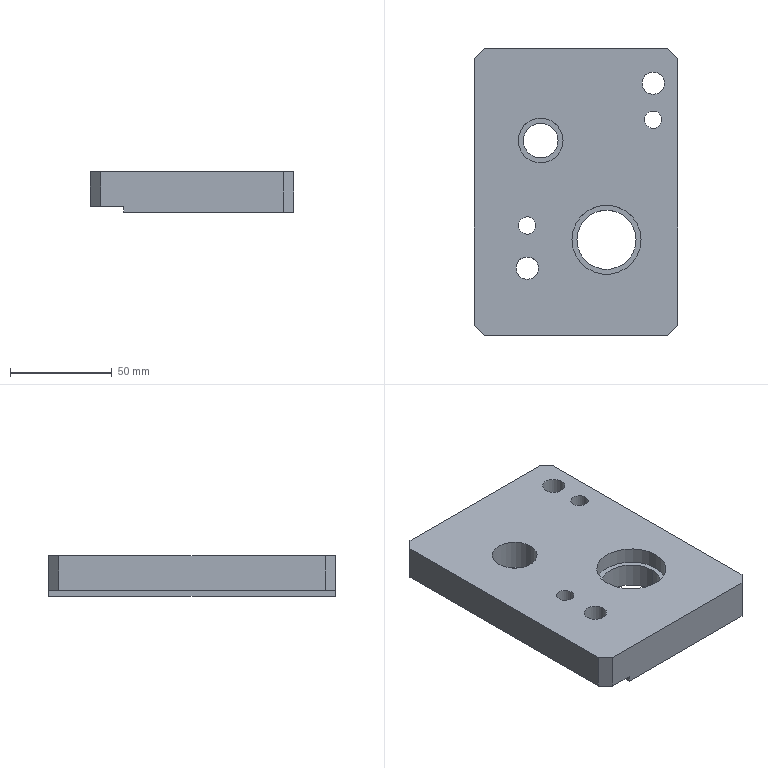Part | STEP file | lll_id3050_x_t | 1 solid | 32 faces | box 100 x 141 x 20 mm | volume 242474 mm3 | plane 18 | cylinder 14 | commonest cylinder face diameters 11 x4 8.5 x2 17 x2 17.07 x2 29.07 x2 22 x1
STEP:
#1=CARTESIAN_POINT('',(3254.117,-145.288,22.5));
#2=VERTEX_POINT('',#1);
#3=CARTESIAN_POINT('',(3258.367,-145.288,22.5));
#4=DIRECTION('',(0.,0.,1.));
#5=DIRECTION('',(-1.,0.,0.));
#6=AXIS2_PLACEMENT_3D('',#3,#4,#5);
#7=CIRCLE('',#6,4.25);
#8=EDGE_CURVE('',#2,#2,#7,.T.);
#9=ORIENTED_EDGE('',*,*,#8,.F.);
#10=EDGE_LOOP('',(#9));
#11=FACE_BOUND('',#10,.T.);
#12=CARTESIAN_POINT('',(3192.117,-197.288,22.5));
#13=VERTEX_POINT('',#12);
#14=CARTESIAN_POINT('',(3196.367,-197.288,22.5));
#15=DIRECTION('',(0.,0.,1.));
#16=DIRECTION('',(-1.,0.,0.));
#17=AXIS2_PLACEMENT_3D('',#14,#15,#16);
#18=CIRCLE('',#17,4.25);
#19=EDGE_CURVE('',#13,#13,#18,.T.);
#20=ORIENTED_EDGE('',*,*,#19,.F.);
#21=EDGE_LOOP('',(#20));
#22=FACE_BOUND('',#21,.T.);
#23=CARTESIAN_POINT('',(3252.867,-127.288,22.5));
#24=VERTEX_POINT('',#23);
#25=CARTESIAN_POINT('',(3258.367,-127.288,22.5));
#26=DIRECTION('',(0.,0.,1.));
#27=DIRECTION('',(-1.,0.,0.));
#28=AXIS2_PLACEMENT_3D('',#25,#26,#27);
#29=CIRCLE('',#28,5.5);
#30=EDGE_CURVE('',#24,#24,#29,.T.);
#31=ORIENTED_EDGE('',*,*,#30,.F.);
#32=EDGE_LOOP('',(#31));
#33=FACE_BOUND('',#32,.T.);
#34=CARTESIAN_POINT('',(3175.367,-110.288,22.5));
#35=VERTEX_POINT('',#34);
#36=CARTESIAN_POINT('',(3265.367,-110.288,22.5));
#37=VERTEX_POINT('',#36);
#38=CARTESIAN_POINT('',(3227.867,-110.288,22.5));
#39=DIRECTION('',(1.,0.,0.));
#40=VECTOR('',#39,1.);
#41=LINE('',#38,#40);
#42=EDGE_CURVE('',#35,#37,#41,.T.);
#43=ORIENTED_EDGE('',*,*,#42,.F.);
#44=CARTESIAN_POINT('',(3170.367,-115.288,22.5));
#45=VERTEX_POINT('',#44);
#46=CARTESIAN_POINT('',(3328.404,42.749,22.5));
#47=DIRECTION('',(-0.7071,-0.7071,0.));
#48=VECTOR('',#47,1.);
#49=LINE('',#46,#48);
#50=EDGE_CURVE('',#35,#45,#49,.T.);
#51=ORIENTED_EDGE('',*,*,#50,.T.);
#52=CARTESIAN_POINT('',(3170.367,-246.288,22.5));
#53=VERTEX_POINT('',#52);
#54=CARTESIAN_POINT('',(3170.367,-166.13,22.5));
#55=DIRECTION('',(0.,-1.,0.));
#56=VECTOR('',#55,1.);
#57=LINE('',#54,#56);
#58=EDGE_CURVE('',#45,#53,#57,.T.);
#59=ORIENTED_EDGE('',*,*,#58,.T.);
#60=CARTESIAN_POINT('',(3175.367,-251.288,22.5));
#61=VERTEX_POINT('',#60);
#62=CARTESIAN_POINT('',(3313.747,-389.668,22.5));
#63=DIRECTION('',(0.7071,-0.7071,0.));
#64=VECTOR('',#63,1.);
#65=LINE('',#62,#64);
#66=EDGE_CURVE('',#53,#61,#65,.T.);
#67=ORIENTED_EDGE('',*,*,#66,.T.);
#68=CARTESIAN_POINT('',(3265.367,-251.288,22.5));
#69=VERTEX_POINT('',#68);
#70=CARTESIAN_POINT('',(3227.867,-251.288,22.5));
#71=DIRECTION('',(-1.,0.,0.));
#72=VECTOR('',#71,1.);
#73=LINE('',#70,#72);
#74=EDGE_CURVE('',#69,#61,#73,.T.);
#75=ORIENTED_EDGE('',*,*,#74,.F.);
#76=CARTESIAN_POINT('',(3270.367,-246.288,22.5));
#77=VERTEX_POINT('',#76);
#78=CARTESIAN_POINT('',(3443.904,-72.751,22.5));
#79=DIRECTION('',(0.7071,0.7071,0.));
#80=VECTOR('',#79,1.);
#81=LINE('',#78,#80);
#82=EDGE_CURVE('',#69,#77,#81,.T.);
#83=ORIENTED_EDGE('',*,*,#82,.T.);
#84=CARTESIAN_POINT('',(3270.367,-115.288,22.5));
#85=VERTEX_POINT('',#84);
#86=CARTESIAN_POINT('',(3270.367,-195.288,22.5));
#87=DIRECTION('',(0.,-1.,0.));
#88=VECTOR('',#87,1.);
#89=LINE('',#86,#88);
#90=EDGE_CURVE('',#85,#77,#89,.T.);
#91=ORIENTED_EDGE('',*,*,#90,.F.);
#92=CARTESIAN_POINT('',(3429.247,-274.168,22.5));
#93=DIRECTION('',(-0.7071,0.7071,0.));
#94=VECTOR('',#93,1.);
#95=LINE('',#92,#94);
#96=EDGE_CURVE('',#85,#37,#95,.T.);
#97=ORIENTED_EDGE('',*,*,#96,.T.);
#98=EDGE_LOOP('',(#43,#51,#59,#67,#75,#83,#91,#97));
#99=FACE_BOUND('',#98,.T.);
#100=CARTESIAN_POINT('',(3190.867,-218.288,22.5));
#101=VERTEX_POINT('',#100);
#102=CARTESIAN_POINT('',(3196.367,-218.288,22.5));
#103=DIRECTION('',(0.,0.,1.));
#104=DIRECTION('',(-1.,0.,0.));
#105=AXIS2_PLACEMENT_3D('',#102,#103,#104);
#106=CIRCLE('',#105,5.5);
#107=EDGE_CURVE('',#101,#101,#106,.T.);
#108=ORIENTED_EDGE('',*,*,#107,.F.);
#109=EDGE_LOOP('',(#108));
#110=FACE_BOUND('',#109,.T.);
#111=CARTESIAN_POINT('',(3214.,-155.5,22.5));
#112=VERTEX_POINT('',#111);
#113=CARTESIAN_POINT('',(3203.,-155.5,22.5));
#114=DIRECTION('',(0.,0.,1.));
#115=DIRECTION('',(1.,0.,0.));
#116=AXIS2_PLACEMENT_3D('',#113,#114,#115);
#117=CIRCLE('',#116,11.);
#118=EDGE_CURVE('',#112,#112,#117,.T.);
#119=ORIENTED_EDGE('',*,*,#118,.F.);
#120=EDGE_LOOP('',(#119));
#121=FACE_BOUND('',#120,.T.);
#122=CARTESIAN_POINT('',(3252.367,-204.288,22.5));
#123=VERTEX_POINT('',#122);
#124=CARTESIAN_POINT('',(3235.367,-204.288,22.5));
#125=DIRECTION('',(0.,0.,-1.));
#126=DIRECTION('',(1.,0.,0.));
#127=AXIS2_PLACEMENT_3D('',#124,#125,#126);
#128=CIRCLE('',#127,17.);
#129=EDGE_CURVE('',#123,#123,#128,.T.);
#130=ORIENTED_EDGE('',*,*,#129,.T.);
#131=EDGE_LOOP('',(#130));
#132=FACE_BOUND('',#131,.T.);
#133=CARTESIAN_POINT('',(3537.284,-166.13,22.5));
#134=DIRECTION('',(0.,0.,1.));
#135=DIRECTION('',(0.,1.,0.));
#136=AXIS2_PLACEMENT_3D('',#133,#134,#135);
#137=PLANE('',#136);
#138=ADVANCED_FACE('',(#11,#22,#33,#99,#110,#121,#132),#137,.T.);
#139=CARTESIAN_POINT('',(3190.867,-197.288,2.5));
#140=VERTEX_POINT('',#139);
#141=CARTESIAN_POINT('',(3196.367,-197.288,2.5));
#142=DIRECTION('',(0.,0.,1.));
#143=DIRECTION('',(-1.,0.,0.));
#144=AXIS2_PLACEMENT_3D('',#141,#142,#143);
#145=CIRCLE('',#144,5.5);
#146=EDGE_CURVE('',#140,#140,#145,.T.);
#147=ORIENTED_EDGE('',*,*,#146,.T.);
#148=EDGE_LOOP('',(#147));
#149=FACE_BOUND('',#148,.T.);
#150=CARTESIAN_POINT('',(3187.867,-218.288,2.5));
#151=VERTEX_POINT('',#150);
#152=CARTESIAN_POINT('',(3196.367,-218.288,2.5));
#153=DIRECTION('',(0.,0.,1.));
#154=DIRECTION('',(-1.,0.,0.));
#155=AXIS2_PLACEMENT_3D('',#152,#153,#154);
#156=CIRCLE('',#155,8.5);
#157=EDGE_CURVE('',#151,#151,#156,.T.);
#158=ORIENTED_EDGE('',*,*,#157,.T.);
#159=EDGE_LOOP('',(#158));
#160=FACE_BOUND('',#159,.T.);
#161=CARTESIAN_POINT('',(3211.535,-155.5,2.5));
#162=VERTEX_POINT('',#161);
#163=CARTESIAN_POINT('',(3194.465,-155.5,2.5));
#164=VERTEX_POINT('',#163);
#165=CARTESIAN_POINT('',(3203.,-155.5,2.5));
#166=DIRECTION('',(0.,0.,-1.));
#167=DIRECTION('',(-1.,0.,0.));
#168=AXIS2_PLACEMENT_3D('',#165,#166,#167);
#169=CIRCLE('',#168,8.535);
#170=EDGE_CURVE('',#162,#164,#169,.T.);
#171=ORIENTED_EDGE('',*,*,#170,.F.);
#172=CARTESIAN_POINT('',(3203.,-155.5,2.5));
#173=DIRECTION('',(0.,0.,-1.));
#174=DIRECTION('',(-1.,0.,0.));
#175=AXIS2_PLACEMENT_3D('',#172,#173,#174);
#176=CIRCLE('',#175,8.535);
#177=EDGE_CURVE('',#164,#162,#176,.T.);
#178=ORIENTED_EDGE('',*,*,#177,.F.);
#179=EDGE_LOOP('',(#171,#178));
#180=FACE_BOUND('',#179,.T.);
#181=CARTESIAN_POINT('',(3249.902,-204.288,2.5));
#182=VERTEX_POINT('',#181);
#183=CARTESIAN_POINT('',(3220.832,-204.288,2.5));
#184=VERTEX_POINT('',#183);
#185=CARTESIAN_POINT('',(3235.367,-204.288,2.5));
#186=DIRECTION('',(0.,0.,-1.));
#187=DIRECTION('',(-1.,0.,0.));
#188=AXIS2_PLACEMENT_3D('',#185,#186,#187);
#189=CIRCLE('',#188,14.535);
#190=EDGE_CURVE('',#182,#184,#189,.T.);
#191=ORIENTED_EDGE('',*,*,#190,.F.);
#192=CARTESIAN_POINT('',(3235.367,-204.288,2.5));
#193=DIRECTION('',(0.,0.,-1.));
#194=DIRECTION('',(-1.,0.,0.));
#195=AXIS2_PLACEMENT_3D('',#192,#193,#194);
#196=CIRCLE('',#195,14.535);
#197=EDGE_CURVE('',#184,#182,#196,.T.);
#198=ORIENTED_EDGE('',*,*,#197,.F.);
#199=EDGE_LOOP('',(#191,#198));
#200=FACE_BOUND('',#199,.T.);
#201=CARTESIAN_POINT('',(3249.867,-127.288,2.5));
#202=VERTEX_POINT('',#201);
#203=CARTESIAN_POINT('',(3258.367,-127.288,2.5));
#204=DIRECTION('',(0.,0.,-1.));
#205=DIRECTION('',(-1.,0.,0.));
#206=AXIS2_PLACEMENT_3D('',#203,#204,#205);
#207=CIRCLE('',#206,8.5);
#208=EDGE_CURVE('',#202,#202,#207,.T.);
#209=ORIENTED_EDGE('',*,*,#208,.F.);
#210=EDGE_LOOP('',(#209));
#211=FACE_BOUND('',#210,.T.);
#212=CARTESIAN_POINT('',(3252.867,-145.288,2.5));
#213=VERTEX_POINT('',#212);
#214=CARTESIAN_POINT('',(3258.367,-145.288,2.5));
#215=DIRECTION('',(0.,0.,-1.));
#216=DIRECTION('',(-1.,0.,0.));
#217=AXIS2_PLACEMENT_3D('',#214,#215,#216);
#218=CIRCLE('',#217,5.5);
#219=EDGE_CURVE('',#213,#213,#218,.T.);
#220=ORIENTED_EDGE('',*,*,#219,.F.);
#221=EDGE_LOOP('',(#220));
#222=FACE_BOUND('',#221,.T.);
#223=CARTESIAN_POINT('',(3265.367,-110.288,2.5));
#224=VERTEX_POINT('',#223);
#225=CARTESIAN_POINT('',(3186.89,-110.288,2.5));
#226=VERTEX_POINT('',#225);
#227=CARTESIAN_POINT('',(2132.435,-110.288,2.5));
#228=DIRECTION('',(-1.,0.,0.));
#229=VECTOR('',#228,1.);
#230=LINE('',#227,#229);
#231=EDGE_CURVE('',#224,#226,#230,.T.);
#232=ORIENTED_EDGE('',*,*,#231,.F.);
#233=CARTESIAN_POINT('',(3270.367,-115.288,2.5));
#234=VERTEX_POINT('',#233);
#235=CARTESIAN_POINT('',(3270.367,-115.288,2.5));
#236=DIRECTION('',(0.7071,-0.7071,0.));
#237=VECTOR('',#236,1.);
#238=LINE('',#235,#237);
#239=EDGE_CURVE('',#224,#234,#238,.T.);
#240=ORIENTED_EDGE('',*,*,#239,.T.);
#241=CARTESIAN_POINT('',(3270.367,-246.288,2.5));
#242=VERTEX_POINT('',#241);
#243=CARTESIAN_POINT('',(3270.367,0.,2.5));
#244=DIRECTION('',(0.,1.,0.));
#245=VECTOR('',#244,1.);
#246=LINE('',#243,#245);
#247=EDGE_CURVE('',#242,#234,#246,.T.);
#248=ORIENTED_EDGE('',*,*,#247,.F.);
#249=CARTESIAN_POINT('',(3265.367,-251.288,2.5));
#250=VERTEX_POINT('',#249);
#251=CARTESIAN_POINT('',(3265.367,-251.288,2.5));
#252=DIRECTION('',(-0.7071,-0.7071,0.));
#253=VECTOR('',#252,1.);
#254=LINE('',#251,#253);
#255=EDGE_CURVE('',#242,#250,#254,.T.);
#256=ORIENTED_EDGE('',*,*,#255,.T.);
#257=CARTESIAN_POINT('',(3186.89,-251.288,2.5));
#258=VERTEX_POINT('',#257);
#259=CARTESIAN_POINT('',(2132.435,-251.288,2.5));
#260=DIRECTION('',(1.,0.,0.));
#261=VECTOR('',#260,1.);
#262=LINE('',#259,#261);
#263=EDGE_CURVE('',#258,#250,#262,.T.);
#264=ORIENTED_EDGE('',*,*,#263,.F.);
#265=CARTESIAN_POINT('',(3186.89,-185.788,2.5));
#266=DIRECTION('',(0.,-1.,0.));
#267=VECTOR('',#266,1.);
#268=LINE('',#265,#267);
#269=EDGE_CURVE('',#226,#258,#268,.T.);
#270=ORIENTED_EDGE('',*,*,#269,.F.);
#271=EDGE_LOOP('',(#232,#240,#248,#256,#264,#270));
#272=FACE_BOUND('',#271,.T.);
#273=CARTESIAN_POINT('',(2132.435,0.,2.5));
#274=DIRECTION('',(0.,0.,-1.));
#275=DIRECTION('',(-1.,0.,0.));
#276=AXIS2_PLACEMENT_3D('',#273,#274,#275);
#277=PLANE('',#276);
#278=ADVANCED_FACE('',(#149,#160,#180,#200,#211,#222,#272),#277,.T.);
#279=CARTESIAN_POINT('',(3190.867,-197.288,9.5));
#280=VERTEX_POINT('',#279);
#281=CARTESIAN_POINT('',(3196.367,-197.288,9.5));
#282=DIRECTION('',(0.,0.,-1.));
#283=DIRECTION('',(-1.,0.,0.));
#284=AXIS2_PLACEMENT_3D('',#281,#282,#283);
#285=CIRCLE('',#284,5.5);
#286=EDGE_CURVE('',#280,#280,#285,.T.);
#287=ORIENTED_EDGE('',*,*,#286,.F.);
#288=EDGE_LOOP('',(#287));
#289=FACE_BOUND('',#288,.T.);
#290=ORIENTED_EDGE('',*,*,#146,.F.);
#291=EDGE_LOOP('',(#290));
#292=FACE_BOUND('',#291,.T.);
#293=CARTESIAN_POINT('',(3196.367,-197.288,-2.5));
#294=DIRECTION('',(0.,0.,1.));
#295=DIRECTION('',(-1.,0.,0.));
#296=AXIS2_PLACEMENT_3D('',#293,#294,#295);
#297=CYLINDRICAL_SURFACE('',#296,5.5);
#298=ADVANCED_FACE('',(#289,#292),#297,.F.);
#299=CARTESIAN_POINT('',(3175.367,-110.288,5.398));
#300=VERTEX_POINT('',#299);
#301=CARTESIAN_POINT('',(3186.89,-110.288,5.398));
#302=VERTEX_POINT('',#301);
#303=CARTESIAN_POINT('',(3227.867,-110.288,5.398));
#304=DIRECTION('',(1.,0.,0.));
#305=VECTOR('',#304,1.);
#306=LINE('',#303,#305);
#307=EDGE_CURVE('',#300,#302,#306,.T.);
#308=ORIENTED_EDGE('',*,*,#307,.F.);
#309=CARTESIAN_POINT('',(3175.367,-110.288,-81.5));
#310=DIRECTION('',(0.,0.,1.));
#311=VECTOR('',#310,1.);
#312=LINE('',#309,#311);
#313=EDGE_CURVE('',#300,#35,#312,.T.);
#314=ORIENTED_EDGE('',*,*,#313,.T.);
#315=ORIENTED_EDGE('',*,*,#42,.T.);
#316=CARTESIAN_POINT('',(3265.367,-110.288,-81.5));
#317=DIRECTION('',(0.,0.,-1.));
#318=VECTOR('',#317,1.);
#319=LINE('',#316,#318);
#320=EDGE_CURVE('',#37,#224,#319,.T.);
#321=ORIENTED_EDGE('',*,*,#320,.T.);
#322=ORIENTED_EDGE('',*,*,#231,.T.);
#323=CARTESIAN_POINT('',(3186.89,-110.288,2.5));
#324=DIRECTION('',(0.,0.,1.));
#325=VECTOR('',#324,1.);
#326=LINE('',#323,#325);
#327=EDGE_CURVE('',#226,#302,#326,.T.);
#328=ORIENTED_EDGE('',*,*,#327,.T.);
#329=EDGE_LOOP('',(#308,#314,#315,#321,#322,#328));
#330=FACE_OUTER_BOUND('',#329,.T.);
#331=CARTESIAN_POINT('',(3227.867,-110.288,-81.5));
#332=DIRECTION('',(0.,1.,0.));
#333=DIRECTION('',(0.,0.,-1.));
#334=AXIS2_PLACEMENT_3D('',#331,#332,#333);
#335=PLANE('',#334);
#336=ADVANCED_FACE('',(#330),#335,.T.);
#337=ORIENTED_EDGE('',*,*,#58,.F.);
#338=CARTESIAN_POINT('',(3170.367,-115.288,5.398));
#339=VERTEX_POINT('',#338);
#340=CARTESIAN_POINT('',(3170.367,-115.288,13.5));
#341=DIRECTION('',(0.,0.,-1.));
#342=VECTOR('',#341,1.);
#343=LINE('',#340,#342);
#344=EDGE_CURVE('',#45,#339,#343,.T.);
#345=ORIENTED_EDGE('',*,*,#344,.T.);
#346=CARTESIAN_POINT('',(3170.367,-246.288,5.398));
#347=VERTEX_POINT('',#346);
#348=CARTESIAN_POINT('',(3170.367,-195.288,5.398));
#349=DIRECTION('',(0.,1.,0.));
#350=VECTOR('',#349,1.);
#351=LINE('',#348,#350);
#352=EDGE_CURVE('',#347,#339,#351,.T.);
#353=ORIENTED_EDGE('',*,*,#352,.F.);
#354=CARTESIAN_POINT('',(3170.367,-246.288,13.5));
#355=DIRECTION('',(0.,0.,1.));
#356=VECTOR('',#355,1.);
#357=LINE('',#354,#356);
#358=EDGE_CURVE('',#347,#53,#357,.T.);
#359=ORIENTED_EDGE('',*,*,#358,.T.);
#360=EDGE_LOOP('',(#337,#345,#353,#359));
#361=FACE_OUTER_BOUND('',#360,.T.);
#362=CARTESIAN_POINT('',(3170.367,-195.288,13.5));
#363=DIRECTION('',(-1.,0.,0.));
#364=DIRECTION('',(0.,0.,1.));
#365=AXIS2_PLACEMENT_3D('',#362,#363,#364);
#366=PLANE('',#365);
#367=ADVANCED_FACE('',(#361),#366,.T.);
#368=ORIENTED_EDGE('',*,*,#263,.T.);
#369=CARTESIAN_POINT('',(3265.367,-251.288,-81.5));
#370=DIRECTION('',(0.,0.,1.));
#371=VECTOR('',#370,1.);
#372=LINE('',#369,#371);
#373=EDGE_CURVE('',#250,#69,#372,.T.);
#374=ORIENTED_EDGE('',*,*,#373,.T.);
#375=ORIENTED_EDGE('',*,*,#74,.T.);
#376=CARTESIAN_POINT('',(3175.367,-251.288,5.398));
#377=VERTEX_POINT('',#376);
#378=CARTESIAN_POINT('',(3175.367,-251.288,-81.5));
#379=DIRECTION('',(0.,0.,-1.));
#380=VECTOR('',#379,1.);
#381=LINE('',#378,#380);
#382=EDGE_CURVE('',#61,#377,#381,.T.);
#383=ORIENTED_EDGE('',*,*,#382,.T.);
#384=CARTESIAN_POINT('',(3186.89,-251.288,5.398));
#385=VERTEX_POINT('',#384);
#386=CARTESIAN_POINT('',(3227.867,-251.288,5.398));
#387=DIRECTION('',(-1.,0.,0.));
#388=VECTOR('',#387,1.);
#389=LINE('',#386,#388);
#390=EDGE_CURVE('',#385,#377,#389,.T.);
#391=ORIENTED_EDGE('',*,*,#390,.F.);
#392=CARTESIAN_POINT('',(3186.89,-251.288,-81.5));
#393=DIRECTION('',(0.,0.,1.));
#394=VECTOR('',#393,1.);
#395=LINE('',#392,#394);
#396=EDGE_CURVE('',#258,#385,#395,.T.);
#397=ORIENTED_EDGE('',*,*,#396,.F.);
#398=EDGE_LOOP('',(#368,#374,#375,#383,#391,#397));
#399=FACE_OUTER_BOUND('',#398,.T.);
#400=CARTESIAN_POINT('',(3227.867,-251.288,-81.5));
#401=DIRECTION('',(0.,-1.,0.));
#402=DIRECTION('',(0.,0.,1.));
#403=AXIS2_PLACEMENT_3D('',#400,#401,#402);
#404=PLANE('',#403);
#405=ADVANCED_FACE('',(#399),#404,.T.);
#406=CARTESIAN_POINT('',(3187.867,-218.288,14.5));
#407=VERTEX_POINT('',#406);
#408=CARTESIAN_POINT('',(3196.367,-218.288,14.5));
#409=DIRECTION('',(0.,0.,-1.));
#410=DIRECTION('',(-1.,0.,0.));
#411=AXIS2_PLACEMENT_3D('',#408,#409,#410);
#412=CIRCLE('',#411,8.5);
#413=EDGE_CURVE('',#407,#407,#412,.T.);
#414=ORIENTED_EDGE('',*,*,#413,.F.);
#415=EDGE_LOOP('',(#414));
#416=FACE_BOUND('',#415,.T.);
#417=ORIENTED_EDGE('',*,*,#157,.F.);
#418=EDGE_LOOP('',(#417));
#419=FACE_BOUND('',#418,.T.);
#420=CARTESIAN_POINT('',(3196.367,-218.288,-2.5));
#421=DIRECTION('',(0.,0.,1.));
#422=DIRECTION('',(0.,1.,0.));
#423=AXIS2_PLACEMENT_3D('',#420,#421,#422);
#424=CYLINDRICAL_SURFACE('',#423,8.5);
#425=ADVANCED_FACE('',(#416,#419),#424,.F.);
#426=CARTESIAN_POINT('',(3192.117,-197.288,9.5));
#427=VERTEX_POINT('',#426);
#428=CARTESIAN_POINT('',(3196.367,-197.288,9.5));
#429=DIRECTION('',(0.,0.,-1.));
#430=DIRECTION('',(-1.,0.,0.));
#431=AXIS2_PLACEMENT_3D('',#428,#429,#430);
#432=CIRCLE('',#431,4.25);
#433=EDGE_CURVE('',#427,#427,#432,.T.);
#434=ORIENTED_EDGE('',*,*,#433,.F.);
#435=EDGE_LOOP('',(#434));
#436=FACE_BOUND('',#435,.T.);
#437=ORIENTED_EDGE('',*,*,#286,.T.);
#438=EDGE_LOOP('',(#437));
#439=FACE_BOUND('',#438,.T.);
#440=CARTESIAN_POINT('',(3196.367,-197.288,9.5));
#441=DIRECTION('',(0.,0.,1.));
#442=DIRECTION('',(-1.,0.,0.));
#443=AXIS2_PLACEMENT_3D('',#440,#441,#442);
#444=PLANE('',#443);
#445=ADVANCED_FACE('',(#436,#439),#444,.F.);
#446=CARTESIAN_POINT('',(3252.867,-127.288,14.5));
#447=VERTEX_POINT('',#446);
#448=CARTESIAN_POINT('',(3258.367,-127.288,14.5));
#449=DIRECTION('',(0.,0.,1.));
#450=DIRECTION('',(-1.,0.,0.));
#451=AXIS2_PLACEMENT_3D('',#448,#449,#450);
#452=CIRCLE('',#451,5.5);
#453=EDGE_CURVE('',#447,#447,#452,.T.);
#454=ORIENTED_EDGE('',*,*,#453,.T.);
#455=EDGE_LOOP('',(#454));
#456=FACE_BOUND('',#455,.T.);
#457=CARTESIAN_POINT('',(3249.867,-127.288,14.5));
#458=VERTEX_POINT('',#457);
#459=CARTESIAN_POINT('',(3258.367,-127.288,14.5));
#460=DIRECTION('',(0.,0.,1.));
#461=DIRECTION('',(-1.,0.,0.));
#462=AXIS2_PLACEMENT_3D('',#459,#460,#461);
#463=CIRCLE('',#462,8.5);
#464=EDGE_CURVE('',#458,#458,#463,.T.);
#465=ORIENTED_EDGE('',*,*,#464,.F.);
#466=EDGE_LOOP('',(#465));
#467=FACE_BOUND('',#466,.T.);
#468=CARTESIAN_POINT('',(3258.367,-127.288,14.5));
#469=DIRECTION('',(0.,0.,1.));
#470=DIRECTION('',(0.,-1.,0.));
#471=AXIS2_PLACEMENT_3D('',#468,#469,#470);
#472=PLANE('',#471);
#473=ADVANCED_FACE('',(#456,#467),#472,.F.);
#474=CARTESIAN_POINT('',(3190.867,-218.288,14.5));
#475=VERTEX_POINT('',#474);
#476=CARTESIAN_POINT('',(3196.367,-218.288,14.5));
#477=DIRECTION('',(0.,0.,-1.));
#478=DIRECTION('',(-1.,0.,0.));
#479=AXIS2_PLACEMENT_3D('',#476,#477,#478);
#480=CIRCLE('',#479,5.5);
#481=EDGE_CURVE('',#475,#475,#480,.T.);
#482=ORIENTED_EDGE('',*,*,#481,.F.);
#483=EDGE_LOOP('',(#482));
#484=FACE_BOUND('',#483,.T.);
#485=ORIENTED_EDGE('',*,*,#413,.T.);
#486=EDGE_LOOP('',(#485));
#487=FACE_BOUND('',#486,.T.);
#488=CARTESIAN_POINT('',(3196.367,-218.288,14.5));
#489=DIRECTION('',(0.,0.,1.));
#490=DIRECTION('',(0.,1.,0.));
#491=AXIS2_PLACEMENT_3D('',#488,#489,#490);
#492=PLANE('',#491);
#493=ADVANCED_FACE('',(#484,#487),#492,.F.);
#494=ORIENTED_EDGE('',*,*,#107,.T.);
#495=EDGE_LOOP('',(#494));
#496=FACE_BOUND('',#495,.T.);
#497=ORIENTED_EDGE('',*,*,#481,.T.);
#498=EDGE_LOOP('',(#497));
#499=FACE_BOUND('',#498,.T.);
#500=CARTESIAN_POINT('',(3196.367,-218.288,97.5));
#501=DIRECTION('',(0.,0.,1.));
#502=DIRECTION('',(0.,1.,0.));
#503=AXIS2_PLACEMENT_3D('',#500,#501,#502);
#504=CYLINDRICAL_SURFACE('',#503,5.5);
#505=ADVANCED_FACE('',(#496,#499),#504,.F.);
#506=ORIENTED_EDGE('',*,*,#464,.T.);
#507=EDGE_LOOP('',(#506));
#508=FACE_BOUND('',#507,.T.);
#509=ORIENTED_EDGE('',*,*,#208,.T.);
#510=EDGE_LOOP('',(#509));
#511=FACE_BOUND('',#510,.T.);
#512=CARTESIAN_POINT('',(3258.367,-127.288,-2.5));
#513=DIRECTION('',(0.,0.,1.));
#514=DIRECTION('',(0.,-1.,0.));
#515=AXIS2_PLACEMENT_3D('',#512,#513,#514);
#516=CYLINDRICAL_SURFACE('',#515,8.5);
#517=ADVANCED_FACE('',(#508,#511),#516,.F.);
#518=ORIENTED_EDGE('',*,*,#247,.T.);
#519=CARTESIAN_POINT('',(3270.367,-115.288,-81.5));
#520=DIRECTION('',(0.,0.,1.));
#521=VECTOR('',#520,1.);
#522=LINE('',#519,#521);
#523=EDGE_CURVE('',#234,#85,#522,.T.);
#524=ORIENTED_EDGE('',*,*,#523,.T.);
#525=ORIENTED_EDGE('',*,*,#90,.T.);
#526=CARTESIAN_POINT('',(3270.367,-246.288,-81.5));
#527=DIRECTION('',(0.,0.,-1.));
#528=VECTOR('',#527,1.);
#529=LINE('',#526,#528);
#530=EDGE_CURVE('',#77,#242,#529,.T.);
#531=ORIENTED_EDGE('',*,*,#530,.T.);
#532=EDGE_LOOP('',(#518,#524,#525,#531));
#533=FACE_OUTER_BOUND('',#532,.T.);
#534=CARTESIAN_POINT('',(3270.367,-195.288,-81.5));
#535=DIRECTION('',(1.,0.,0.));
#536=DIRECTION('',(0.,0.,-1.));
#537=AXIS2_PLACEMENT_3D('',#534,#535,#536);
#538=PLANE('',#537);
#539=ADVANCED_FACE('',(#533),#538,.T.);
#540=ORIENTED_EDGE('',*,*,#30,.T.);
#541=EDGE_LOOP('',(#540));
#542=FACE_BOUND('',#541,.T.);
#543=ORIENTED_EDGE('',*,*,#453,.F.);
#544=EDGE_LOOP('',(#543));
#545=FACE_BOUND('',#544,.T.);
#546=CARTESIAN_POINT('',(3258.367,-127.288,97.5));
#547=DIRECTION('',(0.,0.,1.));
#548=DIRECTION('',(0.,-1.,0.));
#549=AXIS2_PLACEMENT_3D('',#546,#547,#548);
#550=CYLINDRICAL_SURFACE('',#549,5.5);
#551=ADVANCED_FACE('',(#542,#545),#550,.F.);
#552=ORIENTED_EDGE('',*,*,#19,.T.);
#553=EDGE_LOOP('',(#552));
#554=FACE_BOUND('',#553,.T.);
#555=ORIENTED_EDGE('',*,*,#433,.T.);
#556=EDGE_LOOP('',(#555));
#557=FACE_BOUND('',#556,.T.);
#558=CARTESIAN_POINT('',(3196.367,-197.288,97.5));
#559=DIRECTION('',(0.,0.,1.));
#560=DIRECTION('',(-1.,0.,0.));
#561=AXIS2_PLACEMENT_3D('',#558,#559,#560);
#562=CYLINDRICAL_SURFACE('',#561,4.25);
#563=ADVANCED_FACE('',(#554,#557),#562,.F.);
#564=ORIENTED_EDGE('',*,*,#8,.T.);
#565=EDGE_LOOP('',(#564));
#566=FACE_BOUND('',#565,.T.);
#567=CARTESIAN_POINT('',(3254.117,-145.288,9.5));
#568=VERTEX_POINT('',#567);
#569=CARTESIAN_POINT('',(3258.367,-145.288,9.5));
#570=DIRECTION('',(0.,0.,-1.));
#571=DIRECTION('',(-1.,0.,0.));
#572=AXIS2_PLACEMENT_3D('',#569,#570,#571);
#573=CIRCLE('',#572,4.25);
#574=EDGE_CURVE('',#568,#568,#573,.T.);
#575=ORIENTED_EDGE('',*,*,#574,.T.);
#576=EDGE_LOOP('',(#575));
#577=FACE_BOUND('',#576,.T.);
#578=CARTESIAN_POINT('',(3258.367,-145.288,97.5));
#579=DIRECTION('',(0.,0.,1.));
#580=DIRECTION('',(1.,0.,0.));
#581=AXIS2_PLACEMENT_3D('',#578,#579,#580);
#582=CYLINDRICAL_SURFACE('',#581,4.25);
#583=ADVANCED_FACE('',(#566,#577),#582,.F.);
#584=ORIENTED_EDGE('',*,*,#574,.F.);
#585=EDGE_LOOP('',(#584));
#586=FACE_BOUND('',#585,.T.);
#587=CARTESIAN_POINT('',(3252.867,-145.288,9.5));
#588=VERTEX_POINT('',#587);
#589=CARTESIAN_POINT('',(3258.367,-145.288,9.5));
#590=DIRECTION('',(0.,0.,-1.));
#591=DIRECTION('',(-1.,0.,0.));
#592=AXIS2_PLACEMENT_3D('',#589,#590,#591);
#593=CIRCLE('',#592,5.5);
#594=EDGE_CURVE('',#588,#588,#593,.T.);
#595=ORIENTED_EDGE('',*,*,#594,.T.);
#596=EDGE_LOOP('',(#595));
#597=FACE_BOUND('',#596,.T.);
#598=CARTESIAN_POINT('',(3258.367,-145.288,9.5));
#599=DIRECTION('',(0.,0.,1.));
#600=DIRECTION('',(1.,0.,0.));
#601=AXIS2_PLACEMENT_3D('',#598,#599,#600);
#602=PLANE('',#601);
#603=ADVANCED_FACE('',(#586,#597),#602,.F.);
#604=ORIENTED_EDGE('',*,*,#594,.F.);
#605=EDGE_LOOP('',(#604));
#606=FACE_BOUND('',#605,.T.);
#607=ORIENTED_EDGE('',*,*,#219,.T.);
#608=EDGE_LOOP('',(#607));
#609=FACE_BOUND('',#608,.T.);
#610=CARTESIAN_POINT('',(3258.367,-145.288,-2.5));
#611=DIRECTION('',(0.,0.,1.));
#612=DIRECTION('',(1.,0.,0.));
#613=AXIS2_PLACEMENT_3D('',#610,#611,#612);
#614=CYLINDRICAL_SURFACE('',#613,5.5);
#615=ADVANCED_FACE('',(#606,#609),#614,.F.);
#616=CARTESIAN_POINT('',(3220.832,-204.288,14.5));
#617=VERTEX_POINT('',#616);
#618=CARTESIAN_POINT('',(3220.832,-204.288,5.));
#619=DIRECTION('',(0.,0.,-1.));
#620=VECTOR('',#619,1.);
#621=LINE('',#618,#620);
#622=EDGE_CURVE('',#617,#184,#621,.T.);
#623=ORIENTED_EDGE('',*,*,#622,.F.);
#624=CARTESIAN_POINT('',(3249.902,-204.288,14.5));
#625=VERTEX_POINT('',#624);
#626=CARTESIAN_POINT('',(3235.367,-204.288,14.5));
#627=DIRECTION('',(0.,0.,1.));
#628=DIRECTION('',(-1.,0.,0.));
#629=AXIS2_PLACEMENT_3D('',#626,#627,#628);
#630=CIRCLE('',#629,14.535);
#631=EDGE_CURVE('',#617,#625,#630,.T.);
#632=ORIENTED_EDGE('',*,*,#631,.T.);
#633=CARTESIAN_POINT('',(3249.902,-204.288,5.));
#634=DIRECTION('',(0.,0.,1.));
#635=VECTOR('',#634,1.);
#636=LINE('',#633,#635);
#637=EDGE_CURVE('',#182,#625,#636,.T.);
#638=ORIENTED_EDGE('',*,*,#637,.F.);
#639=ORIENTED_EDGE('',*,*,#190,.T.);
#640=EDGE_LOOP('',(#623,#632,#638,#639));
#641=FACE_OUTER_BOUND('',#640,.T.);
#642=CARTESIAN_POINT('',(3235.367,-204.288,5.));
#643=DIRECTION('',(0.,0.,-1.));
#644=DIRECTION('',(-1.,0.,0.));
#645=AXIS2_PLACEMENT_3D('',#642,#643,#644);
#646=CYLINDRICAL_SURFACE('',#645,14.535);
#647=ADVANCED_FACE('',(#641),#646,.F.);
#648=ORIENTED_EDGE('',*,*,#637,.T.);
#649=CARTESIAN_POINT('',(3235.367,-204.288,14.5));
#650=DIRECTION('',(0.,0.,1.));
#651=DIRECTION('',(-1.,0.,0.));
#652=AXIS2_PLACEMENT_3D('',#649,#650,#651);
#653=CIRCLE('',#652,14.535);
#654=EDGE_CURVE('',#625,#617,#653,.T.);
#655=ORIENTED_EDGE('',*,*,#654,.T.);
#656=ORIENTED_EDGE('',*,*,#622,.T.);
#657=ORIENTED_EDGE('',*,*,#197,.T.);
#658=EDGE_LOOP('',(#648,#655,#656,#657));
#659=FACE_OUTER_BOUND('',#658,.T.);
#660=CARTESIAN_POINT('',(3235.367,-204.288,5.));
#661=DIRECTION('',(0.,0.,-1.));
#662=DIRECTION('',(-1.,0.,0.));
#663=AXIS2_PLACEMENT_3D('',#660,#661,#662);
#664=CYLINDRICAL_SURFACE('',#663,14.535);
#665=ADVANCED_FACE('',(#659),#664,.F.);
#666=ORIENTED_EDGE('',*,*,#118,.T.);
#667=EDGE_LOOP('',(#666));
#668=FACE_BOUND('',#667,.T.);
#669=CARTESIAN_POINT('',(3192.,-155.5,7.5));
#670=VERTEX_POINT('',#669);
#671=CARTESIAN_POINT('',(3203.,-155.5,7.5));
#672=DIRECTION('',(0.,0.,-1.));
#673=DIRECTION('',(-1.,0.,0.));
#674=AXIS2_PLACEMENT_3D('',#671,#672,#673);
#675=CIRCLE('',#674,11.);
#676=EDGE_CURVE('',#670,#670,#675,.T.);
#677=ORIENTED_EDGE('',*,*,#676,.T.);
#678=EDGE_LOOP('',(#677));
#679=FACE_BOUND('',#678,.T.);
#680=CARTESIAN_POINT('',(3203.,-155.5,38.5));
#681=DIRECTION('',(0.,0.,-1.));
#682=DIRECTION('',(-1.,0.,0.));
#683=AXIS2_PLACEMENT_3D('',#680,#681,#682);
#684=CYLINDRICAL_SURFACE('',#683,11.);
#685=ADVANCED_FACE('',(#668,#679),#684,.F.);
#686=CARTESIAN_POINT('',(3194.465,-155.5,7.5));
#687=VERTEX_POINT('',#686);
#688=CARTESIAN_POINT('',(3194.465,-155.5,2.));
#689=DIRECTION('',(0.,0.,-1.));
#690=VECTOR('',#689,1.);
#691=LINE('',#688,#690);
#692=EDGE_CURVE('',#687,#164,#691,.T.);
#693=ORIENTED_EDGE('',*,*,#692,.F.);
#694=CARTESIAN_POINT('',(3211.535,-155.5,7.5));
#695=VERTEX_POINT('',#694);
#696=CARTESIAN_POINT('',(3203.,-155.5,7.5));
#697=DIRECTION('',(0.,0.,1.));
#698=DIRECTION('',(-1.,0.,0.));
#699=AXIS2_PLACEMENT_3D('',#696,#697,#698);
#700=CIRCLE('',#699,8.535);
#701=EDGE_CURVE('',#687,#695,#700,.T.);
#702=ORIENTED_EDGE('',*,*,#701,.T.);
#703=CARTESIAN_POINT('',(3211.535,-155.5,2.));
#704=DIRECTION('',(0.,0.,1.));
#705=VECTOR('',#704,1.);
#706=LINE('',#703,#705);
#707=EDGE_CURVE('',#162,#695,#706,.T.);
#708=ORIENTED_EDGE('',*,*,#707,.F.);
#709=ORIENTED_EDGE('',*,*,#170,.T.);
#710=EDGE_LOOP('',(#693,#702,#708,#709));
#711=FACE_OUTER_BOUND('',#710,.T.);
#712=CARTESIAN_POINT('',(3203.,-155.5,2.));
#713=DIRECTION('',(0.,0.,-1.));
#714=DIRECTION('',(-1.,0.,0.));
#715=AXIS2_PLACEMENT_3D('',#712,#713,#714);
#716=CYLINDRICAL_SURFACE('',#715,8.535);
#717=ADVANCED_FACE('',(#711),#716,.F.);
#718=ORIENTED_EDGE('',*,*,#707,.T.);
#719=CARTESIAN_POINT('',(3203.,-155.5,7.5));
#720=DIRECTION('',(0.,0.,1.));
#721=DIRECTION('',(-1.,0.,0.));
#722=AXIS2_PLACEMENT_3D('',#719,#720,#721);
#723=CIRCLE('',#722,8.535);
#724=EDGE_CURVE('',#695,#687,#723,.T.);
#725=ORIENTED_EDGE('',*,*,#724,.T.);
#726=ORIENTED_EDGE('',*,*,#692,.T.);
#727=ORIENTED_EDGE('',*,*,#177,.T.);
#728=EDGE_LOOP('',(#718,#725,#726,#727));
#729=FACE_OUTER_BOUND('',#728,.T.);
#730=CARTESIAN_POINT('',(3203.,-155.5,2.));
#731=DIRECTION('',(0.,0.,-1.));
#732=DIRECTION('',(-1.,0.,0.));
#733=AXIS2_PLACEMENT_3D('',#730,#731,#732);
#734=CYLINDRICAL_SURFACE('',#733,8.535);
#735=ADVANCED_FACE('',(#729),#734,.F.);
#736=CARTESIAN_POINT('',(3218.367,-204.288,14.5));
#737=VERTEX_POINT('',#736);
#738=CARTESIAN_POINT('',(3235.367,-204.288,14.5));
#739=DIRECTION('',(0.,0.,1.));
#740=DIRECTION('',(-1.,0.,0.));
#741=AXIS2_PLACEMENT_3D('',#738,#739,#740);
#742=CIRCLE('',#741,17.);
#743=EDGE_CURVE('',#737,#737,#742,.T.);
#744=ORIENTED_EDGE('',*,*,#743,.T.);
#745=EDGE_LOOP('',(#744));
#746=FACE_BOUND('',#745,.T.);
#747=ORIENTED_EDGE('',*,*,#654,.F.);
#748=ORIENTED_EDGE('',*,*,#631,.F.);
#749=EDGE_LOOP('',(#747,#748));
#750=FACE_BOUND('',#749,.T.);
#751=CARTESIAN_POINT('',(3235.367,-204.288,14.5));
#752=DIRECTION('',(0.,0.,-1.));
#753=DIRECTION('',(-1.,0.,0.));
#754=AXIS2_PLACEMENT_3D('',#751,#752,#753);
#755=PLANE('',#754);
#756=ADVANCED_FACE('',(#746,#750),#755,.F.);
#757=ORIENTED_EDGE('',*,*,#129,.F.);
#758=EDGE_LOOP('',(#757));
#759=FACE_BOUND('',#758,.T.);
#760=ORIENTED_EDGE('',*,*,#743,.F.);
#761=EDGE_LOOP('',(#760));
#762=FACE_BOUND('',#761,.T.);
#763=CARTESIAN_POINT('',(3235.367,-204.288,14.5));
#764=DIRECTION('',(0.,0.,1.));
#765=DIRECTION('',(1.,0.,0.));
#766=AXIS2_PLACEMENT_3D('',#763,#764,#765);
#767=CYLINDRICAL_SURFACE('',#766,17.);
#768=ADVANCED_FACE('',(#759,#762),#767,.F.);
#769=ORIENTED_EDGE('',*,*,#676,.F.);
#770=EDGE_LOOP('',(#769));
#771=FACE_BOUND('',#770,.T.);
#772=ORIENTED_EDGE('',*,*,#724,.F.);
#773=ORIENTED_EDGE('',*,*,#701,.F.);
#774=EDGE_LOOP('',(#772,#773));
#775=FACE_BOUND('',#774,.T.);
#776=CARTESIAN_POINT('',(3203.,-155.5,7.5));
#777=DIRECTION('',(0.,0.,-1.));
#778=DIRECTION('',(-1.,0.,0.));
#779=AXIS2_PLACEMENT_3D('',#776,#777,#778);
#780=PLANE('',#779);
#781=ADVANCED_FACE('',(#771,#775),#780,.F.);
#782=ORIENTED_EDGE('',*,*,#352,.T.);
#783=CARTESIAN_POINT('',(3170.367,-115.288,5.398));
#784=DIRECTION('',(0.7071,0.7071,0.));
#785=VECTOR('',#784,1.);
#786=LINE('',#783,#785);
#787=EDGE_CURVE('',#339,#300,#786,.T.);
#788=ORIENTED_EDGE('',*,*,#787,.T.);
#789=ORIENTED_EDGE('',*,*,#307,.T.);
#790=CARTESIAN_POINT('',(3186.89,-185.788,5.398));
#791=DIRECTION('',(0.,1.,0.));
#792=VECTOR('',#791,1.);
#793=LINE('',#790,#792);
#794=EDGE_CURVE('',#385,#302,#793,.T.);
#795=ORIENTED_EDGE('',*,*,#794,.F.);
#796=ORIENTED_EDGE('',*,*,#390,.T.);
#797=CARTESIAN_POINT('',(3175.367,-251.288,5.398));
#798=DIRECTION('',(-0.7071,0.7071,0.));
#799=VECTOR('',#798,1.);
#800=LINE('',#797,#799);
#801=EDGE_CURVE('',#377,#347,#800,.T.);
#802=ORIENTED_EDGE('',*,*,#801,.T.);
#803=EDGE_LOOP('',(#782,#788,#789,#795,#796,#802));
#804=FACE_OUTER_BOUND('',#803,.T.);
#805=CARTESIAN_POINT('',(3178.628,-185.788,5.398));
#806=DIRECTION('',(0.,0.,1.));
#807=DIRECTION('',(1.,0.,0.));
#808=AXIS2_PLACEMENT_3D('',#805,#806,#807);
#809=PLANE('',#808);
#810=ADVANCED_FACE('',(#804),#809,.F.);
#811=ORIENTED_EDGE('',*,*,#269,.T.);
#812=ORIENTED_EDGE('',*,*,#396,.T.);
#813=ORIENTED_EDGE('',*,*,#794,.T.);
#814=ORIENTED_EDGE('',*,*,#327,.F.);
#815=EDGE_LOOP('',(#811,#812,#813,#814));
#816=FACE_OUTER_BOUND('',#815,.T.);
#817=CARTESIAN_POINT('',(3186.89,-185.788,2.5));
#818=DIRECTION('',(1.,0.,0.));
#819=DIRECTION('',(0.,0.,-1.));
#820=AXIS2_PLACEMENT_3D('',#817,#818,#819);
#821=PLANE('',#820);
#822=ADVANCED_FACE('',(#816),#821,.F.);
#823=ORIENTED_EDGE('',*,*,#50,.F.);
#824=ORIENTED_EDGE('',*,*,#313,.F.);
#825=ORIENTED_EDGE('',*,*,#787,.F.);
#826=ORIENTED_EDGE('',*,*,#344,.F.);
#827=EDGE_LOOP('',(#823,#824,#825,#826));
#828=FACE_OUTER_BOUND('',#827,.T.);
#829=CARTESIAN_POINT('',(3170.367,-115.288,13.5));
#830=DIRECTION('',(0.7071,-0.7071,0.));
#831=DIRECTION('',(0.,0.,1.));
#832=AXIS2_PLACEMENT_3D('',#829,#830,#831);
#833=PLANE('',#832);
#834=ADVANCED_FACE('',(#828),#833,.F.);
#835=ORIENTED_EDGE('',*,*,#239,.F.);
#836=ORIENTED_EDGE('',*,*,#320,.F.);
#837=ORIENTED_EDGE('',*,*,#96,.F.);
#838=ORIENTED_EDGE('',*,*,#523,.F.);
#839=EDGE_LOOP('',(#835,#836,#837,#838));
#840=FACE_OUTER_BOUND('',#839,.T.);
#841=CARTESIAN_POINT('',(3270.367,-115.288,-81.5));
#842=DIRECTION('',(-0.7071,-0.7071,0.));
#843=DIRECTION('',(0.,0.,-1.));
#844=AXIS2_PLACEMENT_3D('',#841,#842,#843);
#845=PLANE('',#844);
#846=ADVANCED_FACE('',(#840),#845,.F.);
#847=ORIENTED_EDGE('',*,*,#255,.F.);
#848=ORIENTED_EDGE('',*,*,#530,.F.);
#849=ORIENTED_EDGE('',*,*,#82,.F.);
#850=ORIENTED_EDGE('',*,*,#373,.F.);
#851=EDGE_LOOP('',(#847,#848,#849,#850));
#852=FACE_OUTER_BOUND('',#851,.T.);
#853=CARTESIAN_POINT('',(3265.367,-251.288,-81.5));
#854=DIRECTION('',(-0.7071,0.7071,0.));
#855=DIRECTION('',(0.,0.,-1.));
#856=AXIS2_PLACEMENT_3D('',#853,#854,#855);
#857=PLANE('',#856);
#858=ADVANCED_FACE('',(#852),#857,.F.);
#859=ORIENTED_EDGE('',*,*,#66,.F.);
#860=ORIENTED_EDGE('',*,*,#358,.F.);
#861=ORIENTED_EDGE('',*,*,#801,.F.);
#862=ORIENTED_EDGE('',*,*,#382,.F.);
#863=EDGE_LOOP('',(#859,#860,#861,#862));
#864=FACE_OUTER_BOUND('',#863,.T.);
#865=CARTESIAN_POINT('',(3175.367,-251.288,-81.5));
#866=DIRECTION('',(0.7071,0.7071,0.));
#867=DIRECTION('',(0.,0.,1.));
#868=AXIS2_PLACEMENT_3D('',#865,#866,#867);
#869=PLANE('',#868);
#870=ADVANCED_FACE('',(#864),#869,.F.);
#871=CLOSED_SHELL('',(#138,#278,#298,#336,#367,#405,#425,#445,#473,#493,#505,#517,#539,#551,#563,#583,#603,#615,#647,#665,#685,#717,#735,#756,#768,#781,#810,#822,#834,#846,#858,#870));
#872=MANIFOLD_SOLID_BREP('',#871);
#873=(LENGTH_UNIT()NAMED_UNIT(*)SI_UNIT(.MILLI.,.METRE.));
#874=UNCERTAINTY_MEASURE_WITH_UNIT(LENGTH_MEASURE(0.00002),#873,'','');
#875=(NAMED_UNIT(*)PLANE_ANGLE_UNIT()SI_UNIT($,.RADIAN.));
#876=PLANE_ANGLE_MEASURE_WITH_UNIT(PLANE_ANGLE_MEASURE(0.01745),#875);
#877=DIMENSIONAL_EXPONENTS(0.,0.,0.,0.,0.,0.,0.);
#878=(CONVERSION_BASED_UNIT('DEGREE',#876)NAMED_UNIT(#877)PLANE_ANGLE_UNIT());
#879=(NAMED_UNIT(*)SI_UNIT($,.STERADIAN.)SOLID_ANGLE_UNIT());
#880=(GEOMETRIC_REPRESENTATION_CONTEXT(3)GLOBAL_UNCERTAINTY_ASSIGNED_CONTEXT((#874))GLOBAL_UNIT_ASSIGNED_CONTEXT((#873,#878,#879))REPRESENTATION_CONTEXT('',''));
#881=ADVANCED_BREP_SHAPE_REPRESENTATION('',(#872),#880);